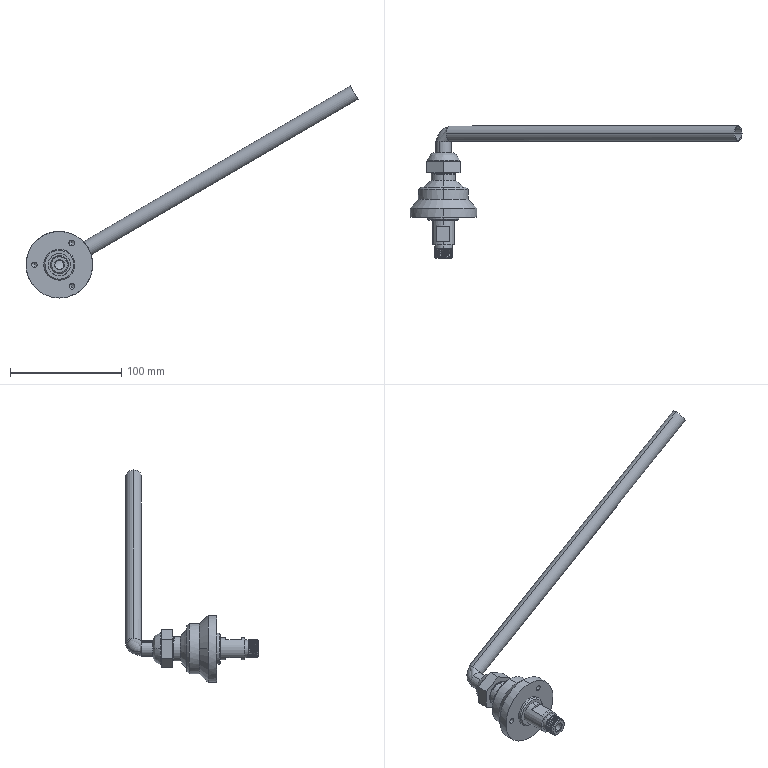Part | NX | features BREP 3 | 3 solids | 131 faces | box 298.662 x 119 x 190.815 mm | volume 92954 mm3 | cylinder 72 | plane 26 | cone 24 | spline 6 | torus 3 | commonest cylinder face diameters 22 x24 16 x18 14 x8 5 x6 12 x4 8 x2